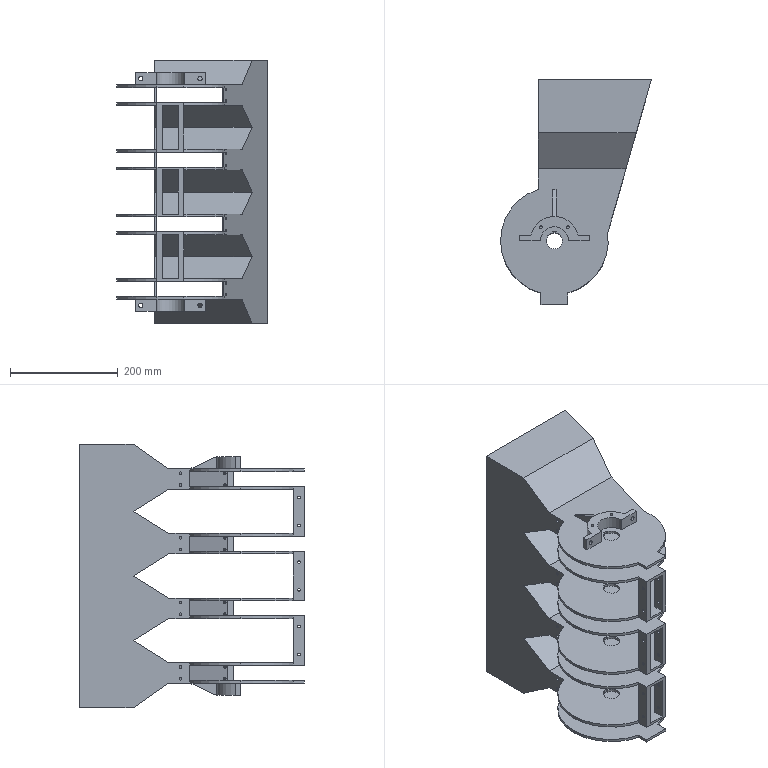Part | SolidWorks | features BaseBody 1 | 1 solid | 234 faces | box 280.198 x 418 x 490 mm | volume 3348300 mm3 | cylinder 136 | plane 98 | commonest cylinder face diameters 5 x64 200 x38 30 x20 8 x8 90 x4 52 x2